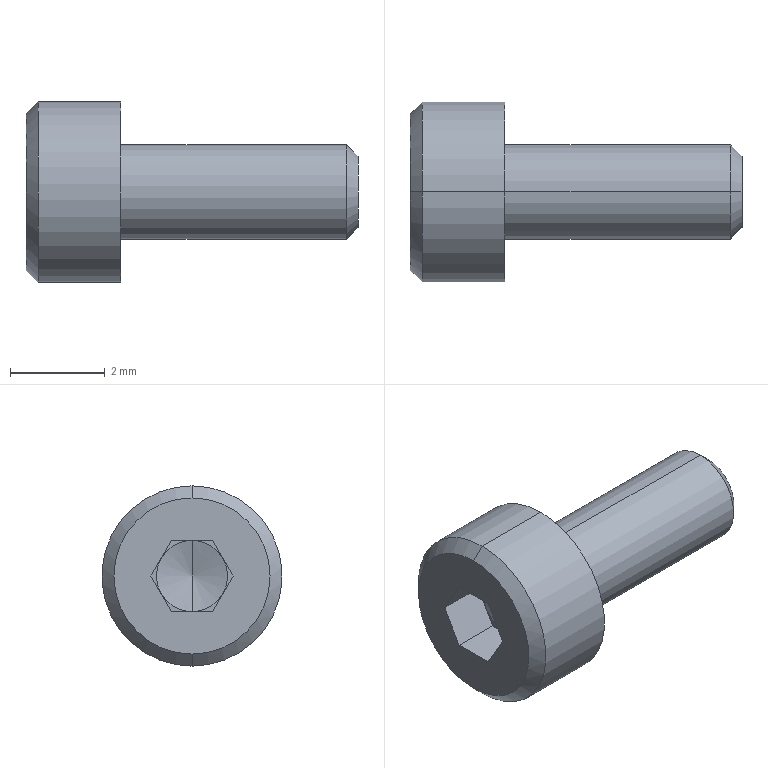Part | SolidWorks | features ICE 1, RevCut 1, Revolution 1 | 1 solid | 25 faces | box 7 x 3.8 x 3.8 mm | volume 35.783 mm3 | plane 15 | cone 6 | cylinder 4 | commonest cylinder face diameters 2 x2 3.8 x2